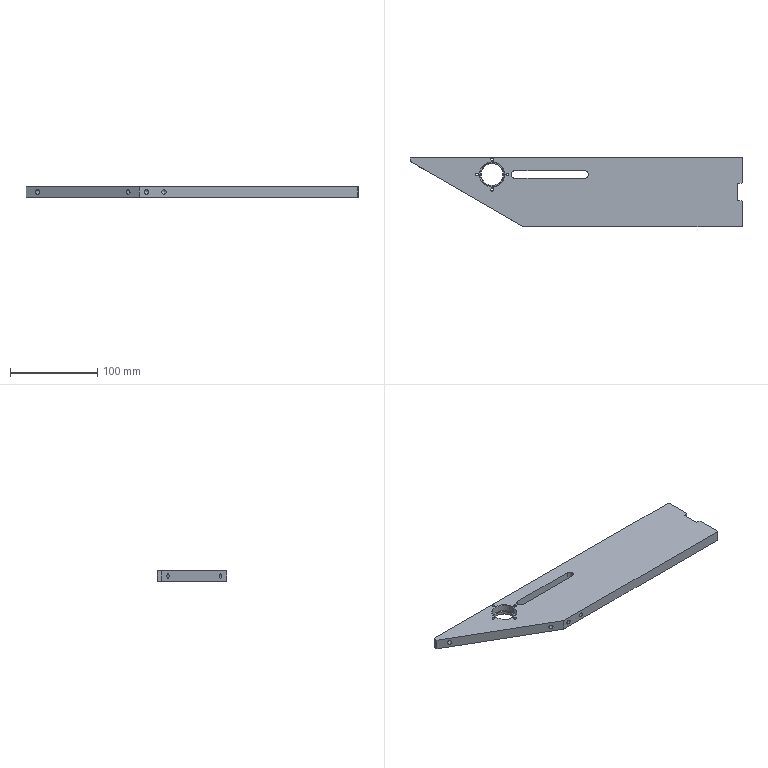NC program | NX | posted with a generic post | part box 380 x 80 x 12 mm
Whole program:
N10 G17 G21 G94 G90
(DRILLING , TOOL : D8A45)
N12 T06 M6
N14 G54
N16 G17 G0 G90 X-96. Y37.5 S3500 M3
N18 G43 Z30. H6
N20 G94 G81 G98 Z-1.75 F250. R3.
N22 X-113.5 Y20.
N24 X-96.
N26 X-78.5
N28 X-96. Y2.5
N30 G80
N32 G0 X-96. Y2.5 Z30.
N34 M5
(DRILLING_COPY , TOOL : 3.3ZT)
N36 T12 M6
N38 G54
N40 G17 G0 G90 X-96. Y37.5 S1500 M3
N42 G43 Z30. H12
N44 G94 G83 G98 Z-14.491 F150. Q2. R3.
N46 X-113.5 Y20.
N48 X-96. Y2.5
N50 X-78.5 Y20.
N52 G80
N54 G0 X-78.5 Y20. Z30.
N56 M5
(ZLEVEL_PROFILE , TOOL : D10)
N58 T04 M6
N60 G54
N62 G17 G0 G90 X189.205 Y49.696 S7000 M3
N64 G43 Z30. H4
N66 Z-1.
N68 G94 G1 X188.786 Y48.131 F1000.
N70 G3 X189.044 Y47.165 R1.
N72 G1 X192.205 Y44.004 F3000.
N74 X192.606 Y43.606
N76 X192.862 Y43.35
N78 X193.029 Y43.175
N80 X193.06 Y43.156
N82 X193.055 Y43.119
N84 X193.019 Y43.11
N86 G2 X195.1 Y39. R5.1
N88 G1 Y11.865
N90 X195.11 Y11.793
N92 X195.042 Y11.769
N94 G2 X193.606 Y7.394 R5.1
N96 G1 X192.606 Y6.394
N98 G2 X190.213 Y5.046 R5.1
N100 G1 X190.1 Y5.022
N102 Y-5.02
N104 G2 X192.606 Y-6.394 R5.1
N106 G1 X193.01 Y-6.797
N108 X193.059 Y-6.839
N110 X193.015 Y-6.887
N112 G2 X195.1 Y-11. R5.1
N114 G1 Y-34.158
N116 X195.097 Y-34.499
N118 Y-43.831
N120 G3 X195.597 Y-44.697 R1.
N122 G1 X197.017 Y-45.517
N124 G0 Z-2.
N126 G1 X195.597 Y-44.697 F1000.
N128 G2 X195.097 Y-43.831 R1.
N130 G1 Y-34.499 F3000.
N132 X195.1 Y-34.158
N134 Y-11.
N136 G3 X193.015 Y-6.887 R5.1
N138 G1 X193.059 Y-6.839
N140 X193.01 Y-6.797
N142 X192.606 Y-6.394
N144 G3 X190.1 Y-5.02 R5.1
N146 G1 Y5.022
N148 X190.213 Y5.046
N150 G3 X192.606 Y6.394 R5.1
N152 G1 X193.606 Y7.394
N154 G3 X195.042 Y11.769 R5.1
N156 G1 X195.11 Y11.793
N158 X195.1 Y11.865
N160 Y39.
N162 G3 X193.019 Y43.11 R5.1
N164 G1 X193.055 Y43.119
N166 X193.06 Y43.156
N168 X193.029 Y43.175
N170 X192.862 Y43.35
N172 X192.606 Y43.606
N174 X192.205 Y44.004
N176 X189.044 Y47.165
N178 G2 X188.786 Y48.131 R1.
N180 G1 X189.205 Y49.696
N182 G0 Z-3.
N184 G1 X188.786 Y48.131 F1000.
N186 G3 X189.044 Y47.165 R1.
N188 G1 X192.205 Y44.004 F3000.
N190 X192.606 Y43.606
N192 X192.862 Y43.35
N194 X193.029 Y43.175
N196 X193.061 Y43.156
N198 X193.055 Y43.119
N200 X193.019 Y43.11
N202 G2 X195.1 Y39. R5.1
N204 G1 Y11.864
N206 X195.11 Y11.793
N208 X195.042 Y11.769
N210 G2 X193.606 Y7.394 R5.1
N212 G1 X192.606 Y6.394
N214 G2 X190.213 Y5.046 R5.1
N216 G1 X190.1 Y5.022
N218 Y-5.02
N220 G2 X192.606 Y-6.394 R5.1
N222 G1 X193.01 Y-6.797
N224 X193.059 Y-6.839
N226 X193.015 Y-6.887
N228 G2 X195.1 Y-11. R5.1
N230 G1 Y-34.158
N232 X195.097 Y-34.499
N234 Y-43.831
N236 G3 X195.597 Y-44.697 R1.
N238 G1 X197.018 Y-45.517
N240 G0 Z-4.
N242 G1 X195.598 Y-44.697 F1000.
N244 G2 X195.098 Y-43.831 R1.
N246 G1 Y-34.499 F3000.
N248 X195.1 Y-34.158
N250 Y-11.
N252 G3 X193.015 Y-6.887 R5.1
N254 G1 X193.059 Y-6.839
N256 X193.01 Y-6.797
N258 X192.606 Y-6.394
N260 G3 X190.1 Y-5.02 R5.1
N262 G1 Y5.022
N264 X190.213 Y5.046
N266 G3 X192.606 Y6.394 R5.1
N268 G1 X193.606 Y7.394
N270 G3 X195.042 Y11.769 R5.1
N272 G1 X195.11 Y11.793
N274 X195.1 Y11.864
N276 Y39.
N278 G3 X193.019 Y43.11 R5.1
N280 G1 X193.055 Y43.119
N282 X193.061 Y43.156
N284 X193.029 Y43.175
N286 X192.862 Y43.35
N288 X192.606 Y43.606
N290 X192.205 Y44.004
N292 X189.044 Y47.166
N294 G2 X188.786 Y48.132 R1.
N296 G1 X189.205 Y49.696
N298 G0 Y49.697 Z-5.
N300 G1 X188.786 Y48.132 F1000.
N302 G3 X189.045 Y47.166 R1.
N304 G1 X192.205 Y44.004 F3000.
N306 X192.606 Y43.606
N308 X192.862 Y43.35
N310 X193.029 Y43.175
N312 X193.061 Y43.156
N314 X193.055 Y43.119
N316 X193.019 Y43.11
N318 G2 X195.1 Y39. R5.1
N320 G1 Y11.864
N322 X195.11 Y11.792
N324 X195.042 Y11.769
N326 G2 X193.606 Y7.394 R5.1
N328 G1 X192.606 Y6.394
N330 G2 X190.213 Y5.046 R5.1
N332 G1 X190.1 Y5.022
N334 Y-5.02
N336 G2 X192.606 Y-6.394 R5.1
N338 G1 X193.01 Y-6.797
N340 X193.059 Y-6.839
N342 X193.015 Y-6.887
N344 G2 X195.1 Y-11. R5.1
N346 G1 Y-34.158
N348 X195.098 Y-34.499
N350 Y-43.831
N352 G3 X195.598 Y-44.697 R1.
N354 G1 X197.018 Y-45.517
N356 G0 Z-6.
N358 G1 X195.598 Y-44.697 F1000.
N360 G2 X195.098 Y-43.831 R1.
N362 G1 Y-34.499 F3000.
N364 X195.1 Y-34.158
N366 Y-11.
N368 G3 X193.015 Y-6.887 R5.1
N370 G1 X193.059 Y-6.839
N372 X193.01 Y-6.797
N374 X192.606 Y-6.394
N376 G3 X190.1 Y-5.02 R5.1
N378 G1 Y5.022
N380 X190.213 Y5.046
N382 G3 X192.606 Y6.394 R5.1
N384 G1 X193.606 Y7.394
N386 G3 X195.042 Y11.769 R5.1
N388 G1 X195.11 Y11.792
N390 X195.1 Y11.864
N392 Y39.
N394 G3 X193.019 Y43.11 R5.1
N396 G1 X193.055 Y43.119
N398 X193.061 Y43.156
N400 X193.029 Y43.175
N402 X192.862 Y43.35
N404 X192.606 Y43.606
N406 X189.045 Y47.166
N408 G2 X188.786 Y48.132 R1.
N410 G1 X189.205 Y49.697
N412 G0 Z-7.
N414 G1 X188.786 Y48.132 F1000.
N416 G3 X189.045 Y47.166 R1.
N418 G1 X192.606 Y43.606 F3000.
N420 X192.862 Y43.35
N422 X193.029 Y43.175
N424 X193.061 Y43.156
N426 X193.055 Y43.119
N428 X193.019 Y43.11
N430 G2 X195.1 Y39. R5.1
N432 G1 Y11.863
N434 X195.11 Y11.792
N436 X195.042 Y11.769
N438 G2 X193.606 Y7.394 R5.1
N440 G1 X192.606 Y6.394
N442 G2 X190.213 Y5.046 R5.1
N444 G1 X190.1 Y5.022
N446 Y-5.02
N448 G2 X192.606 Y-6.394 R5.1
N450 G1 X193.01 Y-6.797
N452 X193.059 Y-6.839
N454 X193.015 Y-6.887
N456 G2 X195.1 Y-11. R5.1
N458 G1 Y-34.158
N460 X195.098 Y-43.831
N462 G3 X195.598 Y-44.698 R1.
N464 G1 X197.018 Y-45.518
N466 G0 Z-8.
N468 G1 X195.598 Y-44.698 F1000.
N470 G2 X195.098 Y-43.831 R1.
N472 G1 X195.1 Y-34.158 F3000.
N474 Y-11.
N476 G3 X193.015 Y-6.887 R5.1
N478 G1 X193.059 Y-6.839
N480 X193.01 Y-6.797
N482 X192.606 Y-6.394
N484 G3 X190.1 Y-5.02 R5.1
N486 G1 Y5.022
N488 X190.213 Y5.046
N490 G3 X192.606 Y6.394 R5.1
N492 G1 X193.606 Y7.394
N494 G3 X195.042 Y11.769 R5.1
N496 G1 X195.11 Y11.792
N498 X195.1 Y11.863
N500 Y39.
N502 G3 X193.019 Y43.11 R5.1
N504 G1 X193.055 Y43.119
N506 X193.061 Y43.156
N508 X193.029 Y43.175
N510 X192.862 Y43.35
N512 X192.606 Y43.606
N514 X189.045 Y47.166
N516 G2 X188.786 Y48.132 R1.
N518 G1 X189.205 Y49.697
N520 G0 Y49.698 Z-9.
N522 G1 X188.786 Y48.132 F1000.
N524 G3 X189.045 Y47.166 R1.
N526 G1 X192.606 Y43.606 F3000.
N528 X192.862 Y43.35
N530 X193.029 Y43.175
N532 X193.061 Y43.156
N534 X193.055 Y43.119
N536 X193.019 Y43.11
N538 G2 X195.1 Y39. R5.1
N540 G1 Y11.863
N542 X195.11 Y11.792
N544 X195.042 Y11.769
N546 G2 X193.606 Y7.394 R5.1
N548 G1 X192.606 Y6.394
N550 G2 X190.213 Y5.046 R5.1
N552 G1 X190.1 Y5.022
N554 Y-5.02
N556 G2 X192.606 Y-6.394 R5.1
N558 G1 X193.01 Y-6.797
N560 X193.059 Y-6.839
N562 X193.015 Y-6.887
N564 G2 X195.1 Y-11. R5.1
N566 G1 Y-34.158
N568 X195.098 Y-43.831
N570 G3 X195.598 Y-44.698 R1.
N572 G1 X197.019 Y-45.518
N574 G0 Z-10.
N576 G1 X195.599 Y-44.698 F1000.
N578 G2 X195.099 Y-43.831 R1.
N580 G1 X195.1 Y-34.158 F3000.
N582 Y-11.
N584 G3 X193.015 Y-6.887 R5.1
N586 G1 X193.06 Y-6.839
N588 X193.01 Y-6.797
N590 X192.606 Y-6.394
N592 G3 X190.1 Y-5.02 R5.1
N594 G1 Y5.022
N596 X190.213 Y5.046
N598 G3 X192.606 Y6.394 R5.1
N600 G1 X193.606 Y7.394
N602 G3 X195.042 Y11.769 R5.1
N604 G1 X195.11 Y11.792
N606 X195.1 Y11.863
N608 Y39.
N610 G3 X193.019 Y43.11 R5.1
N612 G1 X193.055 Y43.119
N614 X193.061 Y43.156
N616 X193.029 Y43.175
N618 X192.862 Y43.35
N620 X192.606 Y43.606
N622 X189.045 Y47.166
N624 G2 X188.786 Y48.132 R1.
N626 G1 X189.205 Y49.698
N628 G0 Z-11.
N630 G1 X188.786 Y48.132 F1000.
N632 G3 X189.045 Y47.166 R1.
N634 G1 X192.606 Y43.606 F3000.
N636 X192.862 Y43.35
N638 X193.029 Y43.175
N640 X193.061 Y43.156
N642 X193.055 Y43.119
N644 X193.019 Y43.11
N646 G2 X195.1 Y39. R5.1
N648 G1 Y11.833
N650 X195.105 Y11.769
N652 X195.042
N654 G2 X193.606 Y7.394 R5.1
N656 G1 X192.606 Y6.394
N658 G2 X190.213 Y5.046 R5.1
N660 G1 X190.1 Y5.022
N662 Y-5.02
N664 G2 X192.606 Y-6.394 R5.1
N666 G1 X193.01 Y-6.797
N668 X193.06 Y-6.839
N670 X193.015 Y-6.887
N672 G2 X195.1 Y-11. R5.1
N674 G1 Y-34.158
N676 X195.099 Y-43.831
N678 G3 X195.599 Y-44.698 R1.
N680 G1 X197.019 Y-45.518
N682 G0 X197.02 Z-12.
N684 G1 X195.599 Y-44.698 F1000.
N686 G2 X195.099 Y-43.831 R1.
N688 G1 X195.1 Y-34.158 F3000.
N690 Y-11.
N692 G3 X193.015 Y-6.887 R5.1
N694 G1 X193.06 Y-6.839
N696 X193.01 Y-6.798
N698 X192.606 Y-6.394
N700 G3 X190.1 Y-5.02 R5.1
N702 G1 Y5.022
N704 X190.213 Y5.046
N706 G3 X192.606 Y6.394 R5.1
N708 G1 X193.606 Y7.394
N710 G3 X195.042 Y11.769 R5.1
N712 G1 X195.105
N714 X195.1 Y11.833
N716 Y39.
N718 G3 X193.019 Y43.11 R5.1
N720 G1 X193.055 Y43.119
N722 X193.061 Y43.156
N724 X193.029 Y43.176
N726 X192.862 Y43.35
N728 X192.606 Y43.606
N730 X189.045 Y47.166
N732 G2 X188.786 Y48.132 R1.
N734 G1 X189.205 Y49.698
N736 G0 Z30.
N738 X-57.407 Y-49.538
N740 Z-1.
N742 G1 Y-48.017 F1000.
N744 G3 X-57.907 Y-47.151 R1.
N746 G1 X-66.955 Y-41.929 F3000.
N748 X-192.55 Y30.583
N750 G2 X-195.1 Y35. R5.1
N752 G1 Y39.
N754 G2 X-193.198 Y42.973 R5.1
N756 G1 X-193.177 Y43.03
N758 X-192.896 Y43.312
N760 X-192.868 Y43.345
N762 X-192.606 Y43.606
N764 X-192.025 Y44.183
N766 X-189.059 Y47.151
N768 G3 X-188.801 Y48.117 R1.
N770 G1 X-189.221 Y49.685
N772 G0 Z-2.
N774 G1 X-188.801 Y48.117 F1000.
N776 G2 X-189.059 Y47.151 R1.
N778 G1 X-192.025 Y44.183 F3000.
N780 X-192.606 Y43.606
N782 X-192.868 Y43.345
N784 X-192.896 Y43.312
N786 X-193.177 Y43.03
N788 X-193.198 Y42.973
N790 G3 X-195.1 Y39. R5.1
N792 G1 Y35.
N794 G3 X-192.55 Y30.583 R5.1
N796 G1 X-66.927 Y-41.942
N798 X-57.907 Y-47.151
N800 G2 X-57.407 Y-48.017 R1.
N802 G1 Y-49.538
N804 G0 Z-3.
N806 G1 Y-48.017 F1000.
N808 G3 X-57.907 Y-47.151 R1.
N810 G1 X-66.955 Y-41.929 F3000.
N812 X-192.55 Y30.583
N814 G2 X-195.1 Y35. R5.1
N816 G1 Y39.
N818 G2 X-193.198 Y42.973 R5.1
N820 G1 X-193.177 Y43.03
N822 X-192.896 Y43.312
N824 X-192.868 Y43.345
N826 X-192.606 Y43.606
N828 X-192.025 Y44.183
N830 X-189.059 Y47.151
N832 G3 X-188.801 Y48.117 R1.
N834 G1 X-189.221 Y49.685
N836 G0 X-189.222 Z-4.
N838 G1 X-188.801 Y48.117 F1000.
N840 G2 X-189.059 Y47.151 R1.
N842 G1 X-192.025 Y44.183 F3000.
N844 X-192.606 Y43.606
N846 X-192.868 Y43.345
N848 X-192.896 Y43.312
N850 X-193.177 Y43.03
N852 X-193.198 Y42.973
N854 G3 X-195.1 Y39. R5.1
N856 G1 Y35.
N858 G3 X-192.55 Y30.583 R5.1
N860 G1 X-66.928 Y-41.942
N862 X-57.907 Y-47.151
N864 G2 X-57.407 Y-48.017 R1.
N866 G1 Y-49.538
N868 G0 Z-5.
N870 G1 Y-48.017 F1000.
N872 G3 X-57.907 Y-47.151 R1.
N874 G1 X-66.955 Y-41.929 F3000.
N876 X-192.55 Y30.583
N878 G2 X-195.1 Y35. R5.1
N880 G1 Y39.
N882 G2 X-193.198 Y42.973 R5.1
N884 G1 X-193.177 Y43.03
N886 X-192.868 Y43.345
N888 X-192.606 Y43.606
N890 X-192.026 Y44.183
N892 X-189.059 Y47.151
N894 G3 X-188.801 Y48.117 R1.
N896 G1 X-189.222 Y49.686
N898 G0 Z-6.
N900 G1 X-188.801 Y48.117 F1000.
N902 G2 X-189.059 Y47.151 R1.
N904 G1 X-192.026 Y44.184 F3000.
N906 X-192.606 Y43.606
N908 X-192.896 Y43.312
N910 X-193.177 Y43.03
N912 X-193.198 Y42.973
N914 G3 X-195.1 Y39. R5.1
N916 G1 Y35.
N918 G3 X-192.55 Y30.583 R5.1
N920 G1 X-66.928 Y-41.942
N922 X-57.907 Y-47.151
N924 G2 X-57.407 Y-48.017 R1.
N926 G1 Y-49.538
N928 G0 Z-7.
N930 G1 Y-48.017 F1000.
N932 G3 X-57.907 Y-47.151 R1.
N934 G1 X-66.955 Y-41.929 F3000.
N936 X-192.55 Y30.583
N938 G2 X-195.1 Y35. R5.1
N940 G1 Y39.
N942 G2 X-193.198 Y42.973 R5.1
N944 G1 X-193.177 Y43.03
N946 X-192.868 Y43.345
N948 X-192.606 Y43.606
N950 X-192.026 Y44.184
N952 X-189.06 Y47.151
N954 G3 X-188.801 Y48.117 R1.
N956 G1 X-189.222 Y49.686
N958 G0 X-189.221 Y49.687 Z-8.
N960 G1 X-188.801 Y48.117 F1000.
N962 G2 X-189.06 Y47.151 R1.
N964 G1 X-192.606 Y43.606 F3000.
N966 X-192.896 Y43.312
N968 X-193.177 Y43.03
N970 X-193.198 Y42.973
N972 G3 X-195.1 Y39. R5.1
N974 G1 Y35.
N976 G3 X-192.55 Y30.583 R5.1
N978 G1 X-66.955 Y-41.929
N980 X-57.907 Y-47.151
N982 G2 X-57.407 Y-48.017 R1.
N984 G1 Y-49.538
N986 G0 Z-9.
N988 G1 Y-48.017 F1000.
N990 G3 X-57.907 Y-47.151 R1.
N992 G1 X-66.955 Y-41.929 F3000.
N994 X-192.55 Y30.583
N996 G2 X-195.1 Y35. R5.1
N998 G1 Y39.
N1000 G2 X-193.198 Y42.973 R5.1
N1002 G1 X-193.177 Y43.03
N1004 X-192.868 Y43.345
N1006 X-192.606 Y43.606
N1008 X-189.06 Y47.151
N1010 G3 X-188.801 Y48.117 R1.
N1012 G1 X-189.221 Y49.687
N1014 G0 Z-10.
N1016 G1 X-188.801 Y48.117 F1000.
N1018 G2 X-189.06 Y47.152 R1.
N1020 G1 X-192.606 Y43.606 F3000.
N1022 X-192.896 Y43.312
N1024 X-193.177 Y43.03
N1026 X-193.198 Y42.973
N1028 G3 X-195.1 Y39. R5.1
N1030 G1 Y35.
N1032 G3 X-192.55 Y30.583 R5.1
N1034 G1 X-66.955 Y-41.929
N1036 X-57.907 Y-47.152
N1038 G2 X-57.407 Y-48.017 R1.
N1040 G1 Y-49.538
N1042 G0 Z-11.
N1044 G1 Y-48.018 F1000.
N1046 G3 X-57.907 Y-47.152 R1.
N1048 G1 X-66.955 Y-41.929 F3000.
N1050 X-192.55 Y30.583
N1052 G2 X-195.1 Y35. R5.1
N1054 G1 Y39.
N1056 G2 X-193.198 Y42.973 R5.1
N1058 G1 X-193.178 Y43.03
N1060 X-192.868 Y43.345
N1062 X-192.606 Y43.606
N1064 X-189.06 Y47.152
N1066 G3 X-188.801 Y48.117 R1.
N1068 G1 X-189.221 Y49.687
N1070 G0 Z-12.
N1072 G1 X-188.801 Y48.118 F1000.
N1074 G2 X-189.06 Y47.152 R1.
N1076 G1 X-192.606 Y43.606 F3000.
N1078 X-192.896 Y43.312
N1080 X-193.178 Y43.03
N1082 X-193.198 Y42.973
N1084 G3 X-195.1 Y39. R5.1
N1086 G1 Y35.
N1088 G3 X-192.55 Y30.583 R5.1
N1090 G1 X-66.955 Y-41.929
N1092 X-57.907 Y-47.152
N1094 G2 X-57.407 Y-48.018 R1.
N1096 G1 Y-49.538
N1098 G0 Z30.
(ZLEVEL_PROFILE_COPY , TOOL : D10)
N1100 X192.668 Y45.962
N1102 Z-12.
N1104 G1 X192.277 Y44.501 F1000.
N1106 G3 X192.536 Y43.536 R1.
N1108 G1 X193.536 Y42.536
N1110 G2 X195. Y39. R5.
N1112 G1 Y11.
N1114 G2 X193.536 Y7.464 R5.
N1116 G1 X192.536 Y6.464
N1118 G2 X190. Y5.101 R5.
N1120 G1 Y-5.101
N1122 G2 X192.536 Y-6.464 R5.
N1124 G1 X193.536 Y-7.464
N1126 G2 X195. Y-11. R5.
N1128 G1 Y-39.
N1130 G3 X195.5 Y-39.866 R1.
N1132 G1 X196.809 Y-40.622
N1134 G0 Z30.
N1136 X-62.096 Y-46.708
N1138 Z-12.
N1140 G1 Y-45.196
N1142 G3 X-62.596 Y-44.33 R1.
N1144 G1 X-192.5 Y30.67
N1146 G2 X-195. Y35. R5.
N1148 G1 Y39.
N1150 G2 X-193.536 Y42.536 R5.
N1152 G1 X-192.536 Y43.536
N1154 G3 X-192.277 Y44.501 R1.
N1156 G1 X-192.668 Y45.962
N1158 G0 Z30.
(HOLE_MILLING , TOOL : D10)
N1160 X-96. Y20.
N1162 Z0.5
N1164 G3 X-93.775 Y17.775 R2.225 F2000.
N1166 X-91.55 Y20. R2.225
N1168 X-91.55 Y20. Z-0.5 I-4.45 J0.
N1170 X-91.55 Y20. Z-1.5 I-4.45 J0.
N1172 X-91.55 Y20. Z-2.5 I-4.45 J0.
N1174 X-91.55 Y20. Z-3.5 I-4.45 J0.
N1176 X-91.55 Y20. Z-4.5 I-4.45 J0.
N1178 X-91.55 Y20. Z-5.5 I-4.45 J0.
N1180 X-91.55 Y20. Z-6.5 I-4.45 J0.
N1182 X-91.55 Y20. Z-7.5 I-4.45 J0.
N1184 X-100.45 Y20. Z-8. I-4.45 J0.
N1186 X-96. Y15.55 R4.45
N1188 X-100.45 Y20. R-4.45
N1190 X-98.225 Y17.775 R2.225
N1192 X-96. Y20. R2.225
N1194 G0 Z0.5
N1196 G3 X-91.55 Y15.55 R4.45
N1198 X-87.1 Y20. R4.45
N1200 X-87.1 Y20. Z-0.5 I-8.9 J0.
N1202 X-87.1 Y20. Z-1.5 I-8.9 J0.
N1204 X-87.1 Y20. Z-2.5 I-8.9 J0.
N1206 X-87.1 Y20. Z-3.5 I-8.9 J0.
N1208 X-87.1 Y20. Z-4.5 I-8.9 J0.
N1210 X-87.1 Y20. Z-5.5 I-8.9 J0.
N1212 X-87.1 Y20. Z-6.5 I-8.9 J0.
N1214 X-87.1 Y20. Z-7.5 I-8.9 J0.
N1216 X-104.9 Y20. Z-8. I-8.9 J0.
N1218 X-96. Y11.1 R8.9
N1220 X-104.9 Y20. R-8.9
N1222 X-100.45 Y15.55 R4.45
N1224 X-96. Y20. R4.45
N1226 G0 Z30.
(HOLE_MILLING_COPY , TOOL : D10)
N1228 Z-7.5
N1230 G3 X-94.125 Y18.125 R1.875 F1250.
N1232 X-92.25 Y20. R1.875
N1234 X-92.25 Y20. Z-8.5 I-3.75 J0.
N1236 X-92.25 Y20. Z-9.5 I-3.75 J0.
N1238 X-92.25 Y20. Z-10.5 I-3.75 J0.
N1240 X-92.25 Y20. Z-11.5 I-3.75 J0.
N1242 X-99.75 Y20. Z-12. I-3.75 J0.
N1244 X-96. Y16.25 R3.75
N1246 X-99.75 Y20. R-3.75
N1248 X-97.875 Y18.125 R1.875
N1250 X-96. Y20. R1.875
N1252 G0 Z-7.5
N1254 G3 X-92.25 Y16.25 R3.75
N1256 X-88.5 Y20. R3.75
N1258 X-88.5 Y20. Z-8.5 I-7.5 J0.
N1260 X-88.5 Y20. Z-9.5 I-7.5 J0.
N1262 X-88.5 Y20. Z-10.5 I-7.5 J0.
N1264 X-88.5 Y20. Z-11.5 I-7.5 J0.
N1266 X-103.5 Y20. Z-12. I-7.5 J0.
N1268 X-96. Y12.5 R7.5
N1270 X-103.5 Y20. R-7.5
N1272 X-99.75 Y16.25 R3.75
N1274 X-96. Y20. R3.75
N1276 G0 Z30.
N1278 M5
(ZLEVEL_PROFILE_1 , TOOL : D6)
N1280 T02 M6
N1282 G54
N1284 G17 G0 G90 X8.162 Y21.25 S7000 M3
N1286 G43 Z30. H2
N1288 Z1.5
N1290 G94 G1 X-30. Z-0.5 F1000.
N1292 X-70. F1450.
N1294 G3 X-71.25 Y20. R1.25
N1296 X-70. Y18.75 R1.25
N1298 G1 X10.
N1300 G3 X11.25 Y20. R1.25
N1302 X10. Y21.25 R1.25
N1304 G1 X-30.
N1306 X-58.645 Z-1.
N1308 X-70.
N1310 G3 X-71.25 Y20. R1.25
N1312 X-70. Y18.75 R1.25
N1314 G1 X10.
N1316 G3 X11.25 Y20. R1.25
N1318 X10. Y21.25 R1.25
N1320 G1 X-30.
N1322 X-58.645 Z-1.5
N1324 X-70.
N1326 G3 X-71.25 Y20. R1.25
N1328 X-70. Y18.75 R1.25
N1330 G1 X10.
N1332 G3 X11.25 Y20. R1.25
N1334 X10. Y21.25 R1.25
N1336 G1 X-30.
N1338 X-58.645 Z-2.
N1340 X-70.
N1342 G3 X-71.25 Y20. R1.25
N1344 X-70. Y18.75 R1.25
N1346 G1 X10.
N1348 G3 X11.25 Y20. R1.25
N1350 X10. Y21.25 R1.25
N1352 G1 X-30.
N1354 X-58.645 Z-2.5
N1356 X-70.
N1358 G3 X-71.25 Y20. R1.25
N1360 X-70. Y18.75 R1.25
N1362 G1 X10.
N1364 G3 X11.25 Y20. R1.25
N1366 X10. Y21.25 R1.25
N1368 G1 X-30.
N1370 X-58.645 Z-3.
N1372 X-70.
N1374 G3 X-71.25 Y20. R1.25
N1376 X-70. Y18.75 R1.25
N1378 G1 X10.
N1380 G3 X11.25 Y20. R1.25
N1382 X10. Y21.25 R1.25
N1384 G1 X-30.
N1386 X-58.645 Z-3.5
N1388 X-70.
N1390 G3 X-71.25 Y20. R1.25
N1392 X-70. Y18.75 R1.25
N1394 G1 X10.
N1396 G3 X11.25 Y20. R1.25
N1398 X10. Y21.25 R1.25
N1400 G1 X-30.
N1402 X-58.645 Z-4.
N1404 X-70.
N1406 G3 X-71.25 Y20. R1.25
N1408 X-70. Y18.75 R1.25
N1410 G1 X10.
N1412 G3 X11.25 Y20. R1.25
N1414 X10. Y21.25 R1.25
N1416 G1 X-30.
N1418 X-58.645 Z-4.5
N1420 X-70.
N1422 G3 X-71.25 Y20. R1.25
N1424 X-70. Y18.75 R1.25
N1426 G1 X10.
N1428 G3 X11.25 Y20. R1.25
N1430 X10. Y21.25 R1.25
N1432 G1 X-30.
N1434 X-58.645 Z-5.
N1436 X-70.
N1438 G3 X-71.25 Y20. R1.25
N1440 X-70. Y18.75 R1.25
N1442 G1 X10.
N1444 G3 X11.25 Y20. R1.25
N1446 X10. Y21.25 R1.25
N1448 G1 X-30.
N1450 X-58.645 Z-5.5
N1452 X-70.
N1454 G3 X-71.25 Y20. R1.25
N1456 X-70. Y18.75 R1.25
N1458 G1 X10.
N1460 G3 X11.25 Y20. R1.25
N1462 X10. Y21.25 R1.25
N1464 G1 X-30.
N1466 X-58.645 Z-6.
N1468 X-70.
N1470 G3 X-71.25 Y20. R1.25
N1472 X-70. Y18.75 R1.25
N1474 G1 X10.
N1476 G3 X11.25 Y20. R1.25
N1478 X10. Y21.25 R1.25
N1480 G1 X-30.
N1482 X-58.645 Z-6.5
N1484 X-70.
N1486 G3 X-71.25 Y20. R1.25
N1488 X-70. Y18.75 R1.25
N1490 G1 X10.
N1492 G3 X11.25 Y20. R1.25
N1494 X10. Y21.25 R1.25
N1496 G1 X-30.
N1498 X-58.645 Z-7.
N1500 X-70.
N1502 G3 X-71.25 Y20. R1.25
N1504 X-70. Y18.75 R1.25
N1506 G1 X10.
N1508 G3 X11.25 Y20. R1.25
N1510 X10. Y21.25 R1.25
N1512 G1 X-30.
N1514 X-58.645 Z-7.5
N1516 X-70.
N1518 G3 X-71.25 Y20. R1.25
N1520 X-70. Y18.75 R1.25
N1522 G1 X10.
N1524 G3 X11.25 Y20. R1.25
N1526 X10. Y21.25 R1.25
N1528 G1 X-30.
N1530 X-58.645 Z-8.
N1532 X-70.
N1534 G3 X-71.25 Y20. R1.25
N1536 X-70. Y18.75 R1.25
N1538 G1 X10.
N1540 G3 X11.25 Y20. R1.25
N1542 X10. Y21.25 R1.25
N1544 G1 X-30.
N1546 X-58.645 Z-8.5
N1548 X-70.
N1550 G3 X-71.25 Y20. R1.25
N1552 X-70. Y18.75 R1.25
N1554 G1 X10.
N1556 G3 X11.25 Y20. R1.25
N1558 X10. Y21.25 R1.25
N1560 G1 X-30.
N1562 X-58.645 Z-9.
N1564 X-70.
N1566 G3 X-71.25 Y20. R1.25
N1568 X-70. Y18.75 R1.25
N1570 G1 X10.
N1572 G3 X11.25 Y20. R1.25
N1574 X10. Y21.25 R1.25
N1576 G1 X-30.
N1578 X-58.645 Z-9.5
N1580 X-70.
N1582 G3 X-71.25 Y20. R1.25
N1584 X-70. Y18.75 R1.25
N1586 G1 X10.
N1588 G3 X11.25 Y20. R1.25
N1590 X10. Y21.25 R1.25
N1592 G1 X-30.
N1594 X-58.645 Z-10.
N1596 X-70.
N1598 G3 X-71.25 Y20. R1.25
N1600 X-70. Y18.75 R1.25
N1602 G1 X10.
N1604 G3 X11.25 Y20. R1.25
N1606 X10. Y21.25 R1.25
N1608 G1 X-30.
N1610 X-58.645 Z-10.5
N1612 X-70.
N1614 G3 X-71.25 Y20. R1.25
N1616 X-70. Y18.75 R1.25
N1618 G1 X10.
N1620 G3 X11.25 Y20. R1.25
N1622 X10. Y21.25 R1.25
N1624 G1 X-30.
N1626 X-58.645 Z-11.
N1628 X-70.
N1630 G3 X-71.25 Y20. R1.25
N1632 X-70. Y18.75 R1.25
N1634 G1 X10.
N1636 G3 X11.25 Y20. R1.25
N1638 X10. Y21.25 R1.25
N1640 G1 X-30.
N1642 X-58.645 Z-11.5
N1644 X-70.
N1646 G3 X-71.25 Y20. R1.25
N1648 X-70. Y18.75 R1.25
N1650 G1 X10.
N1652 G3 X11.25 Y20. R1.25
N1654 X10. Y21.25 R1.25
N1656 G1 X-30.
N1658 X-58.645 Z-12.
N1660 X-70.
N1662 G3 X-71.25 Y20. R1.25
N1664 X-70. Y18.75 R1.25
N1666 G1 X10.
N1668 G3 X11.25 Y20. R1.25
N1670 X10. Y21.25 R1.25
N1672 G1 X-58.645
N1674 Z-10.5
N1676 G0 Z30.
N1678 M5
(PLANAR_MILL , TOOL : D8A45)
N1680 T06 M6
N1682 G54
N1684 G17 G0 G90 X-95.755 Y2.371 S7000 M3
N1686 G43 Z30. H6
N1688 Z0.
N1690 G94 G1 X-95.75 Y2.626 Z-0.069 F1250.
N1692 X-95.874 Y2.75 Z-0.116
N1694 X-96.067 Z-0.168
N1696 X-96.234 Y2.653 Z-0.22
N1698 Y2.347 Z-0.302
N1700 X-96.016 Y2.22 Z-0.369
N1702 X-95.75 Y2.374 Z-0.452
N1704 Y2.626 Z-0.519
N1706 X-95.874 Y2.75 Z-0.566
N1708 X-96.067 Z-0.618
N1710 X-96.234 Y2.653 Z-0.67
N1712 Y2.347 Z-0.752
N1714 X-96.016 Y2.22 Z-0.819
N1716 X-95.75 Y2.374 Z-0.902
N1718 Y2.626 Z-0.969
N1720 X-95.874 Y2.75 Z-1.016
N1722 X-96.067 Z-1.068
N1724 X-96.234 Y2.653 Z-1.12
N1726 Y2.347 Z-1.202
N1728 X-96.016 Y2.22 Z-1.269
N1730 X-95.75 Y2.374 Z-1.352
N1732 Y2.626 Z-1.419
N1734 X-95.874 Y2.75 Z-1.466
N1736 X-96. Z-1.5
N1738 G3 X-96.25 Y2.5 R0.25
N1740 X-96. Y2.75 R-0.25
N1742 G1 Z0.
N1744 G0 Z30.
N1746 X-113.255 Y19.871
N1748 Z0.
N1750 G1 X-113.25 Y20.126 Z-0.069
N1752 X-113.374 Y20.25 Z-0.116
N1754 X-113.567 Z-0.168
N1756 X-113.734 Y20.153 Z-0.22
N1758 Y19.847 Z-0.302
N1760 X-113.516 Y19.72 Z-0.369
N1762 X-113.25 Y19.874 Z-0.452
N1764 Y20.126 Z-0.519
N1766 X-113.374 Y20.25 Z-0.566
N1768 X-113.567 Z-0.618
N1770 X-113.734 Y20.153 Z-0.67
N1772 Y19.847 Z-0.752
N1774 X-113.516 Y19.72 Z-0.819
N1776 X-113.25 Y19.874 Z-0.902
N1778 Y20.126 Z-0.969
N1780 X-113.374 Y20.25 Z-1.016
N1782 X-113.567 Z-1.068
N1784 X-113.734 Y20.153 Z-1.12
N1786 Y19.847 Z-1.202
N1788 X-113.516 Y19.72 Z-1.269
N1790 X-113.25 Y19.874 Z-1.352
N1792 Y20.126 Z-1.419
N1794 X-113.374 Y20.25 Z-1.466
N1796 X-113.5 Z-1.5
N1798 G3 X-113.75 Y20. R0.25
N1800 X-113.5 Y20.25 R-0.25
N1802 X-113.547 Y19.995 R0.5
N1804 G1 Z0.
N1806 G0 Z30.
N1808 X-95.755 Y37.371
N1810 Z0.
N1812 G1 X-95.75 Y37.626 Z-0.069
N1814 X-95.874 Y37.75 Z-0.116
N1816 X-96.067 Z-0.168
N1818 X-96.234 Y37.653 Z-0.22
N1820 Y37.347 Z-0.302
N1822 X-96.016 Y37.22 Z-0.369
N1824 X-95.75 Y37.374 Z-0.452
N1826 Y37.626 Z-0.519
N1828 X-95.874 Y37.75 Z-0.566
N1830 X-96.067 Z-0.618
N1832 X-96.234 Y37.653 Z-0.67
N1834 Y37.347 Z-0.752
N1836 X-96.016 Y37.22 Z-0.819
N1838 X-95.75 Y37.374 Z-0.902
N1840 Y37.626 Z-0.969
N1842 X-95.874 Y37.75 Z-1.016
N1844 X-96.067 Z-1.068
N1846 X-96.234 Y37.653 Z-1.12
N1848 Y37.347 Z-1.202
N1850 X-96.016 Y37.22 Z-1.269
N1852 X-95.75 Y37.374 Z-1.352
N1854 Y37.626 Z-1.419
N1856 X-95.874 Y37.75 Z-1.466
N1858 X-96. Z-1.5
N1860 G3 X-96.25 Y37.5 R0.25
N1862 X-96. Y37.75 R-0.25
N1864 G1 Z0.
N1866 G0 Z30.
N1868 X-94.437 Y31.393
N1870 Z0.
N1872 G1 Z-1.5
N1874 X-95.134 Y32.6
N1876 G3 X-96. Y33.1 R1.
N1878 X-109.1 Y20. R13.1
N1880 X-96. Y33.1 R-13.1
N1882 X-96.866 Y32.6 R1.
N1884 G1 X-97.563 Y31.393
N1886 Z0.
N1888 G0 Z30.
N1890 X-78.255 Y19.871
N1892 Z0.
N1894 G1 X-78.25 Y20.126 Z-0.069
N1896 X-78.374 Y20.25 Z-0.116
N1898 X-78.567 Z-0.168
N1900 X-78.734 Y20.153 Z-0.22
N1902 Y19.847 Z-0.302
N1904 X-78.516 Y19.72 Z-0.369
N1906 X-78.25 Y19.874 Z-0.452
N1908 Y20.126 Z-0.519
N1910 X-78.374 Y20.25 Z-0.566
N1912 X-78.567 Z-0.618
N1914 X-78.734 Y20.153 Z-0.67
N1916 Y19.847 Z-0.752
N1918 X-78.516 Y19.72 Z-0.819
N1920 X-78.25 Y19.874 Z-0.902
N1922 Y20.126 Z-0.969
N1924 X-78.374 Y20.25 Z-1.016
N1926 X-78.567 Z-1.068
N1928 X-78.734 Y20.153 Z-1.12
N1930 Y19.847 Z-1.202
N1932 X-78.516 Y19.72 Z-1.269
N1934 X-78.25 Y19.874 Z-1.352
N1936 Y20.126 Z-1.419
N1938 X-78.374 Y20.25 Z-1.466
N1940 X-78.5 Z-1.5
N1942 G3 X-78.75 Y20. R0.25
N1944 X-78.5 Y20.25 R-0.25
N1946 X-78.547 Y19.995 R0.5
N1948 G1 Z0.
N1950 G0 Z30.
N1952 X-28.499 Y21.25
N1954 Z0.
N1956 G1 Z-1.5
N1958 X-29.134 Y22.35
N1960 G3 X-30. Y22.85 R1.
N1962 G1 X-70.
N1964 G3 X-72.85 Y20. R2.85
N1966 X-70. Y17.15 R2.85
N1968 G1 X10.
N1970 G3 X12.85 Y20. R2.85
N1972 X10. Y22.85 R2.85
N1974 G1 X-30.
N1976 G3 X-30.866 Y22.35 R1.
N1978 G1 X-31.501 Y21.25
N1980 Z0.
N1982 G0 Z30.
(PLANAR_MILL_COPY , TOOL : D8A45)
N1984 X193. Y40.501
N1986 Z0.
N1988 G1 Z-1.5
N1990 X191.9 Y39.866
N1992 G3 X191.4 Y39. R1.
N1994 G1 Y11.041
N1996 G2 X190.961 Y9.981 R1.5
N1998 G1 X190.019 Y9.039
N2000 G2 X188.959 Y8.6 R1.5
N2002 G1 X186.4
N2004 Y-8.6
N2006 X188.959
N2008 G2 X190.019 Y-9.039 R1.5
N2010 G1 X190.961 Y-9.981
N2012 G2 X191.4 Y-11.041 R1.5
N2014 G1 Y-38.959
N2016 G2 X190.961 Y-40.019 R1.5
N2018 G1 X189.99 Y-40.99
N2020 G3 X189.731 Y-41.956 R1.
N2022 G1 X190.06 Y-43.183
N2024 Z0.
N2026 G0 Z30.
N2028 X-60.296 Y-43.349
N2030 Z0.
N2032 G1 Z-1.5
N2034 Y-42.078
N2036 G3 X-60.796 Y-41.212 R1.
N2038 G1 X-190.65 Y33.759
N2040 G2 X-191.4 Y35.058 R1.5
N2042 G1 Y38.959
N2044 G2 X-190.961 Y40.019 R1.5
N2046 G1 X-189.99 Y40.99
N2048 G3 X-189.731 Y41.956 R1.
N2050 G1 X-190.06 Y43.183
N2052 Z0.
N2054 G0 Z30.
N2056 M5
(刀补4 , TOOL : D10)
N2058 T04 M6
N2060 G54
N2062 G17 G0 G90 X-96. Y20. S7000 M3
N2064 G43 Z30. H4
N2066 Z0.5
N2068 G41 G94 G1 X-90.767 Y17.275 F1000. D4
N2070 G3 X-87.05 Y20. R2.857
N2072 X-87.05 Y20. Z-2.5 I-8.95 J0.
N2074 X-87.05 Y20. Z-5.5 I-8.95 J0.
N2076 X-91.525 Y12.249 Z-8. R-8.95
N2078 X-88.249 Y24.475 R8.95
N2080 X-91.525 Y12.249 R-8.95
N2082 X-91.024 Y16.831 R2.857
N2084 G40
N2086 G1 X-96. Y20.
N2088 G0 Z30.
N2090 M5
N2092 M2